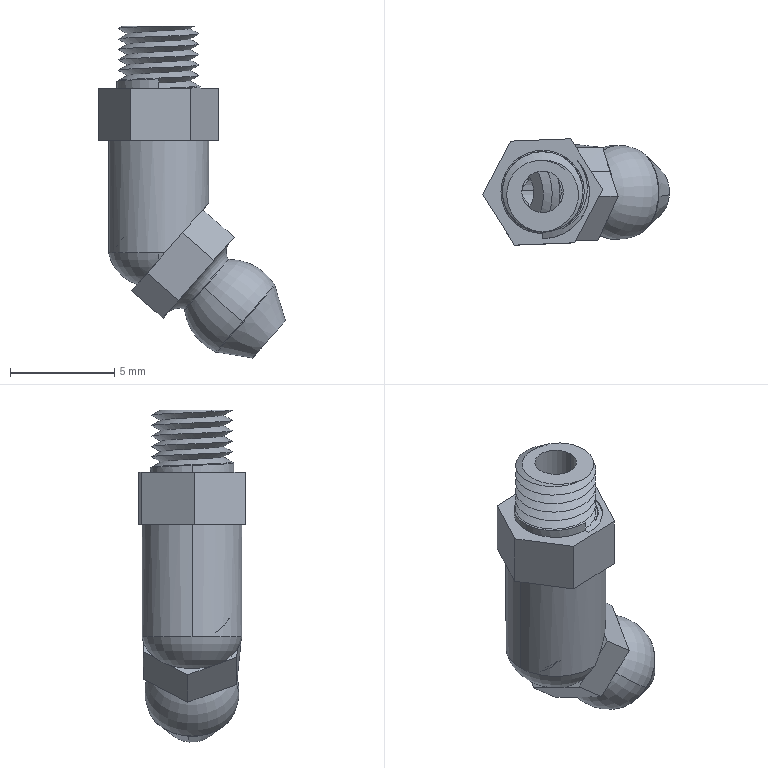Part | SolidWorks | 2 solids | 76 faces | box 8.981 x 5.109 x 15.952 mm | volume 219.147 mm3 | plane 33 | cylinder 17 | torus 11 | cone 8 | spline 7 | commonest cylinder face diameters 2 x6 4 x5 3.3 x2 4.5 x2 4.8 x2